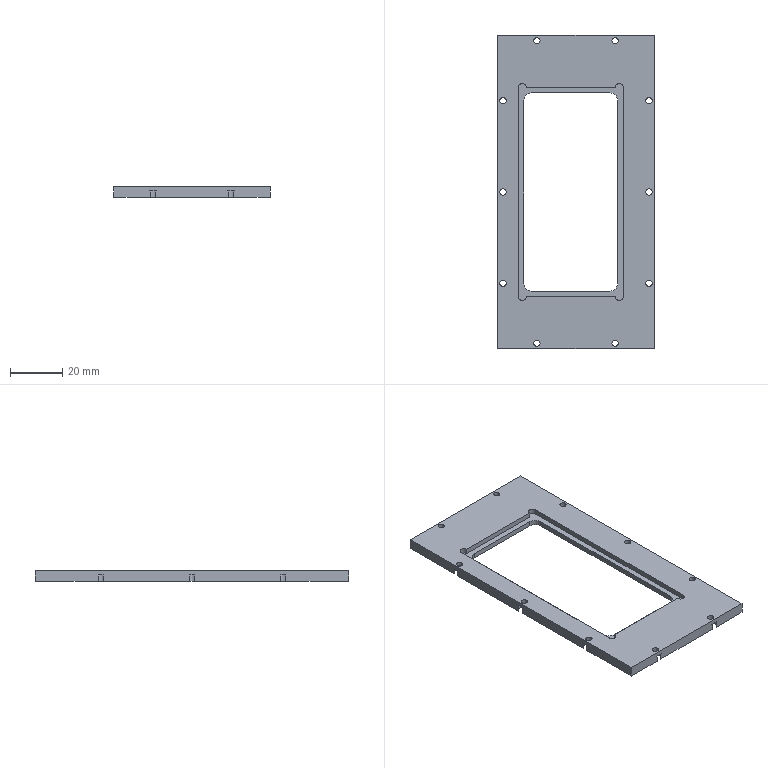Part | SolidWorks | features HoleWzd 4, ICE 3, Extrusion 1, Fillet 1 | 1 solid | 74 faces | box 60 x 120 x 4 mm | volume 16436 mm3 | cylinder 49 | plane 25 | commonest cylinder face diameters 4.4 x21 2.4 x20 3 x4 6 x4